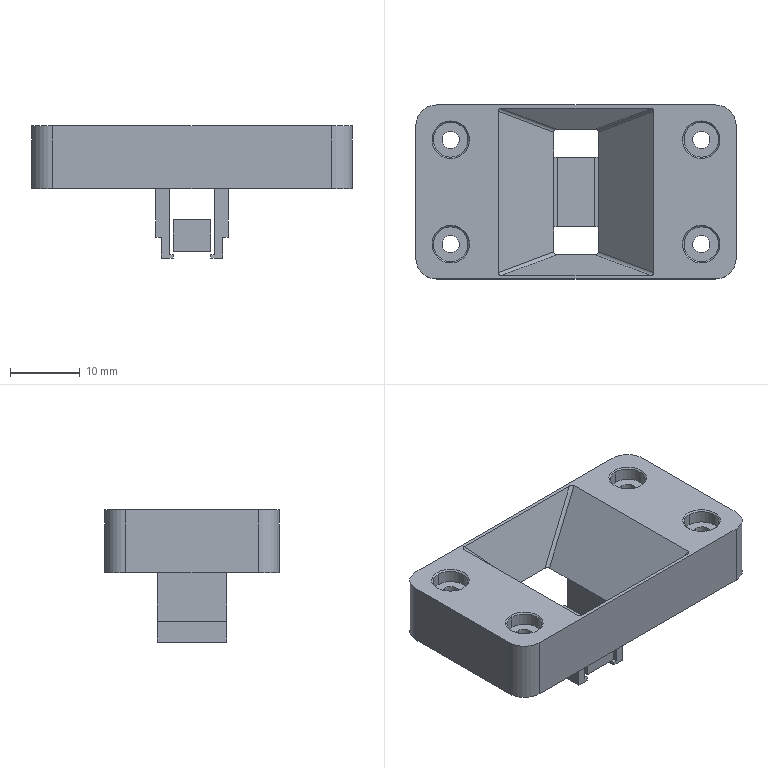NC program | NX | posted with a generic post | part box 46 x 25 x 19 mm
Lines 1 to 1574 of 3737:
N10 G17 G21 G94 G90
(FLOOR_WALL , TOOL : D63)
N12 T01 M6
N14 G54
N16 G17 G0 G90 X-60.5 Y0. S6500 M3
N18 G43 Z30. H1
N20 Z3.
N22 G94 G1 Z0. F1250.
N24 X-57.5
N26 X57.5
N28 X60.5
N30 Z3.
N32 G0 Z30.
N34 M5
(DRILLING_COPY_1 , TOOL : D6A45)
N36 T07 M6
N38 G54
N40 G17 G0 G90 X18. Y-7.5 S5000 M3
N42 G43 Z30. H7
N44 G94 G81 G98 Z-1. F250. R3.
N46 Y7.5
N48 X-18.
N50 Y-7.5
N52 G80
N54 G0 X-18. Y-7.5 Z30.
N56 M5
(DRILLING_COPY_COPY_1 , TOOL : 2.5ZT)
N58 T12 M6
N60 G54
N62 G17 G0 G90 X-18. Y7.5 S2000 M3
N64 G43 Z30. H12
N66 G94 G83 G98 Z-11.251 F120. Q2. R3.
N68 Y-7.5
N70 X18. Y7.5
N72 Y-7.5
N74 G80
N76 G0 X18. Y-7.5 Z30.
N78 M5
(ADAPTIVE_MILLING , TOOL : D10)
N80 T10 M6
N82 G54
N84 G17 G0 G90 X-33.697 Y-0.049 S9500 M3
N86 G43 Z30. H10
N88 Z-18.
N90 G94 G1 Z-19. F1000.
N92 X-32.34 Y-0.579 F3000.
N94 G3 X-31.05 Y-0.049 R1.015
N96 X-30.406 Y3.11 R9.424
N98 X-30.192 Y13.206 R193.319
N100 G2 X-27.283 Y17.541 R6.034
N102 X-21.613 Y19.34 R13.274
N104 X-12.124 Y19.68 R91.439
N106 G1 X-10.224 Y19.685
N108 X-7.224 Y19.689
N110 X0.376 Y19.69
N112 X23.276
N114 X23.376
N116 X23.476 Y19.686
N118 G2 X27.913 Y16.952 R5.88
N120 X29.811 Y11.32 R12.732
N122 X30.174 Y2.832 R75.409
N124 G1 X30.181 Y1.532
N126 X30.186 Y-0.468
N128 X30.189 Y-3.668
N130 X30.191 Y-12.268
N132 Y-12.768
N134 X30.19 Y-12.868
N136 X30.187 Y-12.967
N138 X30.182 Y-13.067
N140 X30.165 Y-13.267
N142 G2 X27.294 Y-17.52 R6.049
N144 X21.631 Y-19.334 R13.161
N146 X12.942 Y-19.676 R82.484
N148 G1 X11.342 Y-19.683
N150 X9.142 Y-19.687
N152 X5.242 Y-19.69
N154 X-17.158
N156 X-23.258
N158 X-23.358
N160 G2 X-27.727 Y-17.211 R5.74
N162 X-29.739 Y-11.833 R11.883
N164 X-30.084 Y-1.654 R57.601
N166 G3 X-29.419 Y10.621 R116.784
N168 G2 X-25.504 Y16.566 R7.722
N170 X-19.339 Y18.47 R15.631
N172 X-9.852 Y18.864 R87.436
N174 G1 X-8.252 Y18.872
N176 X-6.052 Y18.877
N178 X-2.552 Y18.88
N180 X7.048 Y18.882
N182 X20.548
N184 X20.648 Y18.881
N186 G2 X26.926 Y15.19 R7.564
N188 X28.962 Y8.865 R15.122
N190 X29.363 Y-0.521 R83.334
N192 X29.351 Y-10.72 R504.514
N194 X25.37 Y-16.621 R7.723
N196 X18.893 Y-18.518 R16.177
N198 X9.103 Y-18.868 R101.21
N200 G1 X7.603 Y-18.874
N202 X5.203 Y-18.878
N204 X0.903 Y-18.881
N206 X-20.497 Y-18.882
N208 X-20.697 Y-18.88
N210 X-20.897 Y-18.873
N212 G2 X-27.058 Y-14.981 R7.639
N214 X-29.004 Y-8.52 R15.779
N216 X-29.036 Y0.264 R43.131
N218 G3 X-28.648 Y8.654 R335.998
N220 G2 X-27.767 Y11.838 R8.866
N222 X-26.744 Y14.068 R8.11
N224 X-21.539 Y17.498 R8.456
N226 X-7.536 Y18.058 R139.726
N228 G1 X-5.536 Y18.065
N230 X-2.736 Y18.07
N232 X2.064 Y18.072
N234 X18.064 Y18.073
N236 X18.364 Y18.071
N238 X18.564 Y18.067
N240 G2 X21.765 Y17.44 R9.062
N242 X26.801 Y13.982 R8.383
N244 X28.147 Y9.526 R8.782
N246 X28.561 Y-3.864 R168.54
N248 X28.507 Y-8.962 R72.787
N250 X27.952 Y-11.228 R9.275
N252 X24.482 Y-16.301 R8.398
N254 X20.026 Y-17.647 R8.782
N256 X6.436 Y-18.062 R172.59
N258 G1 X4.036 Y-18.068
N260 X0.336 Y-18.072
N262 X-8.664 Y-18.073
N264 X-18.164
N266 X-18.364 Y-18.071
N268 X-18.564 Y-18.067
N270 G2 X-21.77 Y-17.439 R9.081
N272 X-26.801 Y-13.982 R8.381
N274 X-28.147 Y-9.526 R8.782
N276 X-28.15 Y1.332 R71.064
N278 G1 Y9.474
N280 X-28.147 Y9.526
N282 G2 X-27.746 Y11.905 R8.34
N284 G1 X-27.505 Y12.664
N286 X-27.133 Y13.371
N288 X-26.744 Y14.068
N290 X-26.241 Y14.688
N292 X-25.723 Y15.296
N294 X-25.109 Y15.806
N296 X-24.482 Y16.301
N298 X-23.78 Y16.681
N300 X-23.07 Y17.045
N302 X-22.307 Y17.281
N304 X-21.539 Y17.498
N306 X-20.026 Y17.647
N308 X-19.974 Y17.65
N310 X19.974
N312 X20.026 Y17.647
N314 G2 X21.831 Y17.42 R11.605
N316 G1 X22.5 Y17.221
N318 X23.164 Y17.005
N320 X23.871 Y16.633
N322 X24.568 Y16.244
N324 X25.188 Y15.741
N326 X25.796 Y15.223
N328 X26.306 Y14.609
N330 X26.801 Y13.982
N332 X27.181 Y13.28
N334 X27.545 Y12.57
N336 X27.781 Y11.807
N338 X27.998 Y11.039
N340 X28.147 Y9.526
N342 X28.15 Y9.474
N344 Y-9.474
N346 X28.147 Y-9.526
N348 G2 X27.949 Y-11.235 R72.543
N350 G1 X27.736 Y-11.952
N352 X27.505 Y-12.664
N354 X27.133 Y-13.371
N356 X26.744 Y-14.068
N358 X26.241 Y-14.688
N360 X25.723 Y-15.296
N362 X25.109 Y-15.806
N364 X24.482 Y-16.301
N366 X23.78 Y-16.681
N368 X23.07 Y-17.045
N370 X22.307 Y-17.281
N372 X21.539 Y-17.498
N374 X20.026 Y-17.647
N376 X19.974 Y-17.65
N378 X-19.974
N380 X-20.026 Y-17.647
N382 G2 X-21.831 Y-17.42 R11.605
N384 G1 X-22.5 Y-17.221
N386 X-23.164 Y-17.005
N388 X-23.871 Y-16.633
N390 X-24.568 Y-16.244
N392 X-25.188 Y-15.741
N394 X-25.796 Y-15.223
N396 X-26.306 Y-14.609
N398 X-26.801 Y-13.982
N400 X-27.181 Y-13.28
N402 X-27.545 Y-12.57
N404 X-27.781 Y-11.807
N406 X-27.998 Y-11.039
N408 X-28.147 Y-9.526
N410 X-28.15 Y-9.474
N412 Y1.426
N414 G3 X-29.013 Y2.425 R1.016
N416 G1 X-30.593 Y2.657
N418 Z-16.
N420 G0 Z30.
N422 M5
(ZLEVEL_PROFILE_COPY_COPY_1 , TOOL : D10JING)
N424 T11 M6
N426 G54
N428 G17 G0 G90 X-20.841 Y17.958 S9500 M3
N430 G43 Z30. H11
N432 Z-16.
N434 G94 G1 Z-19. F1200.
N436 G3 X-20. Y17.5 R1.
N438 G1 X20.
N440 G2 X28. Y9.5 R8.
N442 G1 Y-9.5
N444 G2 X20. Y-17.5 R8.
N446 G1 X-20.
N448 G2 X-28. Y-9.5 R8.
N450 G1 Y9.5
N452 G2 X-20. Y17.5 R8.
N454 G3 X-19.134 Y18. R1.
N456 G1 Z-16.
N458 G0 Z30.
N460 M5
(FIXED_CONTOUR , TOOL : D6)
N462 T06 M6
N464 G54
N466 G17 G0 G90 X8.757 Y2.485 S9500 M3
N468 G43 Z30. H6
N470 Z3.6
N472 G94 G1 Z0.438 F500.
N474 G3 X8.455 Y1.967 R0.6
N476 G1 X8.43 Y-6.253 Z0.409 F2500.
N478 X8.417 Y-8.89 Z0.395
N480 X8.419 Y-9.033 Z0.413
N482 X8.402 Y-9.043 Z0.444
N484 X4.433 Y-9.042 Z0.441
N486 X-5.767 Y-9.027 Z0.398
N488 X-8.137 Y-9.021 Z0.378
N490 X-8.38 Y-9.016 Z0.364
N492 X-8.377 Y-8.765 Z0.349
N494 X-8.331 Y6.648 Z0.298
N496 X-8.32 Y8.788 Z0.285
N498 X-8.318 Y8.996 Z0.303
N500 X-4.046 Y8.995 Z0.302
N502 X5.501 Y8.981 Z0.259
N504 X8.258 Y8.973 Z0.236
N506 X8.28 Y8.945 Z0.241
N508 X8.233 Y-6.326 Z0.188
N510 X8.221 Y-8.735 Z0.174
N512 X8.214 Y-8.947 Z0.166
N514 X4.808 Y-8.949 Z0.162
N516 X-6.007 Y-8.933 Z0.115
N518 X-8.145 Y-8.927 Z0.097
N520 X-8.181 Y-8.882 Z0.129
N522 X-8.134 Y6.844 Z0.076
N524 X-8.122 Y8.865 Z0.063
N526 X-8.069 Y8.903 Z0.025
N528 X-3.127 Y8.901 Z0.018
N530 X5.301 Y8.888 Z-0.021
N532 X8.03 Y8.878 Z-0.041
N534 X8.083 Y8.818 Z0.018
N536 X8.037 Y-6.324 Z-0.033
N538 X8.024 Y-8.757 Z-0.047
N540 X8.011 Y-8.805 Z-0.062
N542 X7.966 Y-8.854 Z-0.113
N544 X4.278 Y-8.855 Z-0.119
N546 X-5.897 Y-8.84 Z-0.165
N548 X-7.69 Y-8.835 Z-0.18
N550 X-7.913 Y-8.824 Z-0.173
N552 X-7.985 Y-8.745 Z-0.092
N554 X-7.939 Y6.483 Z-0.144
N556 X-7.927 Y8.714 Z-0.157
N558 X-7.834 Y8.809 Z-0.256
N560 X-3.07 Y8.807 Z-0.262
N562 X5.549 Y8.794 Z-0.303
N564 X7.782 Y8.786 Z-0.32
N566 X7.886 Y8.671 Z-0.202
N568 X7.841 Y-6.109 Z-0.253
N570 X7.829 Y-8.564 Z-0.267
N572 X7.818 Y-8.651 Z-0.279
N574 X7.705 Y-8.764 Z-0.393
N576 X2.414 Y-8.76 Z-0.406
N578 X-6.196 Y-8.745 Z-0.448
N580 X-7.54 Y-8.741 Z-0.46
N582 X-7.665 Y-8.73 Z-0.451
N584 X-7.789 Y-8.578 Z-0.312
N586 X-7.739 Y7.085 Z-0.368
N588 X-7.732 Y8.36 Z-0.376
N590 X-7.725 Y8.57 Z-0.384
N592 X-7.581 Y8.716 Z-0.536
N594 X-3.439 Y8.714 Z-0.541
N596 X5.431 Y8.7 Z-0.583
N598 X7.532 Y8.695 Z-0.598
N600 X7.668 Y8.546 Z-0.449
N602 X7.69 Y8.499 Z-0.423
N604 X7.645 Y-6.125 Z-0.475
N606 X7.632 Y-8.458 Z-0.488
N608 X7.618 Y-8.506 Z-0.505
N610 X7.476 Y-8.66 Z-0.664
N612 X7.217 Y-8.67 Z-0.674
N614 X0.537 Y-8.664 Z-0.692
N616 X-6.612 Y-8.651 Z-0.732
N618 X-7.266 Y-8.649 Z-0.738
N620 X-7.417 Y-8.638 Z-0.731
N622 X-7.555 Y-8.486 Z-0.575
N624 X-7.592 Y-8.426 Z-0.533
N626 X-7.542 Y7.225 Z-0.59
N628 X-7.535 Y8.385 Z-0.598
N630 X-7.518 Y8.432 Z-0.617
N632 X-7.379 Y8.583 Z-0.773
N634 X-7.336 Y8.623 Z-0.815
N636 X-3.098 Y8.621 Z-0.822
N638 X5.607 Y8.606 Z-0.865
N640 X7.165 Y8.603 Z-0.876
N642 X7.296 Y8.591 Z-0.867
N644 X7.444 Y8.427 Z-0.7
N646 X7.494 Y8.352 Z-0.644
N648 X7.448 Y-6.076 Z-0.695
N650 X7.435 Y-8.341 Z-0.71
N652 X7.214 Y-8.577 Z-0.952
N654 X0.101 Y-8.57 Z-0.976
N656 X-6.447 Y-8.557 Z-1.012
N658 X-7.125 Y-8.556 Z-1.017
N660 X-7.171 Y-8.543 Z-1.007
N662 X-7.3 Y-8.402 Z-0.862
N664 X-7.396 Y-8.282 Z-0.754
N666 X-7.344 Y7.325 Z-0.812
N668 X-7.339 Y8.248 Z-0.818
N670 X-7.206 Y8.407 Z-0.968
N672 X-7.084 Y8.53 Z-1.095
N674 X-3.316 Y8.528 Z-1.101
N676 X5.401 Y8.513 Z-1.144
N678 X7.035 Y8.51 Z-1.155
N680 X7.298 Y8.222 Z-0.865
N682 X7.25 Y-6.314 Z-0.918
N684 X7.239 Y-8.191 Z-0.931
N686 X7.097 Y-8.346 Z-1.09
N688 X6.961 Y-8.484 Z-1.232
N690 X-1.38 Y-8.474 Z-1.262
N692 X-6.909 Y-8.463 Z-1.296
N694 X-7.166 Y-8.182 Z-1.013
N696 X-7.2 Y-8.132 Z-0.975
N698 X-7.147 Y7.464 Z-1.035
N700 X-7.143 Y8.112 Z-1.039
N702 X-6.86 Y8.418 Z-1.357
N704 X-6.808 Y8.436 Z-1.375
N706 X-2.814 Y8.434 Z-1.384
N708 X5.435 Y8.42 Z-1.425
N710 X6.792 Y8.414 Z-1.434
N712 X7.074 Y8.102 Z-1.117
N714 X7.101 Y8.049 Z-1.086
N716 X7.055 Y-5.998 Z-1.137
N718 X7.043 Y-8.04 Z-1.151
N720 X6.766 Y-8.342 Z-1.463
N722 X6.703 Y-8.391 Z-1.512
N724 X-1.526 Y-8.38 Z-1.544
N726 X-6.462 Y-8.37 Z-1.574
N728 X-6.672 Y-8.362 Z-1.568
N730 X-6.94 Y-8.065 Z-1.267
N732 X-7.004 Y-7.984 Z-1.195
N734 X-6.951 Y7.324 Z-1.255
N736 X-6.947 Y7.961 Z-1.259
N738 X-6.669 Y8.263 Z-1.572
N740 X-6.587 Y8.343 Z-1.655
N742 X-2.976 Y8.34 Z-1.663
N744 X5.308 Y8.326 Z-1.705
N746 X6.498 Y8.323 Z-1.714
N748 X6.556 Y8.308 Z-1.699
N750 X6.905 Y7.922 Z-1.307
N752 X6.858 Y-6.073 Z-1.359
N754 X6.849 Y-7.739 Z-1.369
N756 X6.838 Y-7.9 Z-1.382
N758 X6.545 Y-8.22 Z-1.712
N760 X6.462 Y-8.298 Z-1.791
N762 X-1.462 Y-8.287 Z-1.824
N764 X-6.202 Y-8.277 Z-1.852
N766 X-6.428 Y-8.264 Z-1.843
N768 X-6.67 Y-7.997 Z-1.571
N770 X-6.807 Y-7.837 Z-1.416
N772 X-6.755 Y7.16 Z-1.475
N774 X-6.752 Y7.631 Z-1.478
N776 X-6.745 Y7.817 Z-1.486
N778 X-6.347 Y8.249 Z-1.934
N780 X-2.561 Y8.246 Z-1.945
N782 X5.253 Y8.233 Z-1.985
N784 X6.064 Y8.231 Z-1.991
N786 X6.301 Y8.223 Z-1.986
N788 X6.709 Y7.772 Z-1.528
N790 X6.66 Y-6.35 Z-1.582
N792 X6.653 Y-7.59 Z-1.59
N794 X6.645 Y-7.746 Z-1.598
N796 X6.36 Y-8.056 Z-1.919
N798 X6.215 Y-8.204 Z-2.071
N800 X-2.643 Y-8.191 Z-2.111
N802 X-5.955 Y-8.184 Z-2.131
N804 X-6.175 Y-8.179 Z-2.128
N806 X-6.558 Y-7.753 Z-1.696
N808 X-6.611 Y-7.681 Z-1.637
N810 X-6.559 Y6.99 Z-1.695
N812 X-6.556 Y7.471 Z-1.699
N814 X-6.549 Y7.667 Z-1.707
N816 X-6.132 Y8.119 Z-2.176
N818 X-6.074 Y8.157 Z-2.214
N820 X-1.07 Y8.151 Z-2.232
N822 X5.446 Y8.139 Z-2.268
N824 X5.872 Y8.138 Z-2.271
N826 X6.056 Y8.126 Z-2.261
N828 X6.441 Y7.701 Z-1.828
N830 X6.512 Y7.604 Z-1.749
N832 X6.465 Y-6.029 Z-1.802
N834 X6.456 Y-7.588 Z-1.811
N836 X5.972 Y-8.11 Z-2.353
N838 X-1.594 Y-8.1 Z-2.385
N840 X-5.916 Y-8.091 Z-2.41
N842 X-6.151 Y-7.837 Z-2.155
N844 X-6.29 Y-7.682 Z-1.998
N846 X-6.415 Y-7.531 Z-1.858
N848 X-6.362 Y7. Z-1.917
N850 X-6.359 Y7.509 Z-1.92
N852 X-5.851 Y8.06 Z-2.492
N854 X-1.703 Y8.058 Z-2.509
N856 X5.307 Y8.045 Z-2.547
N858 X5.708 Y8.044 Z-2.551
N860 X5.809 Y8.032 Z-2.539
N862 X6.306 Y7.482 Z-1.98
N864 X6.315 Y7.225 Z-1.97
N866 X6.268 Y-6.118 Z-2.023
N868 X6.261 Y-7.25 Z-2.031
N870 X6.256 Y-7.443 Z-2.037
N872 X5.857 Y-7.875 Z-2.485
N874 X5.711 Y-8.017 Z-2.632
N876 X-3.184 Y-8.003 Z-2.675
N878 X-5.604 Y-7.998 Z-2.689
N880 X-5.685 Y-7.987 Z-2.679
N882 X-6.172 Y-7.446 Z-2.131
N884 X-6.219 Y-7.374 Z-2.078
N886 X-6.165 Y7.165 Z-2.14
N888 X-6.161 Y7.361 Z-2.144
N890 X-5.613 Y7.954 Z-2.76
N892 X-5.562 Y7.97 Z-2.774
N894 X4.043 Y7.955 Z-2.818
N896 X5.524 Y7.951 Z-2.83
N898 X5.575 Y7.924 Z-2.803
N900 X6.058 Y7.39 Z-2.26
N902 X6.12 Y7.303 Z-2.19
N904 X6.071 Y-6.062 Z-2.244
N906 X6.065 Y-7.09 Z-2.251
N908 X6.054 Y-7.298 Z-2.264
N910 X5.514 Y-7.883 Z-2.871
N912 X5.458 Y-7.923 Z-2.913
N914 X-2.94 Y-7.91 Z-2.954
N916 X-5.185 Y-7.906 Z-2.967
N918 X-5.434 Y-7.898 Z-2.962
N920 X-6.023 Y-7.243 Z-2.299
N922 X-5.969 Y7.02 Z-2.36
N924 X-5.965 Y7.21 Z-2.364
N926 X-5.352 Y7.875 Z-3.054
N928 X4.947 Y7.859 Z-3.107
N930 X5.304 Y7.855
N932 X5.923 Y7.166 Z-2.411
N934 X5.874 Y-6.159 Z-2.466
N936 X5.868 Y-7.108 Z-2.473
N938 X5.858 Y-7.148 Z-2.484
N940 X5.255 Y-7.799 Z-3.162
N942 X5.217 Y-7.83 Z-3.193
N944 X-4.705 Y-7.813 Z-3.245
N946 X-4.972 Y-7.812 Z-3.247
N948 X-5.187 Y-7.803 Z-3.239
N950 X-5.826 Y-7.092 Z-2.52
N952 X-5.773 Y6.869 Z-2.58
N954 X-5.765 Y7.065 Z-2.59
N956 X-5.105 Y7.78 Z-3.331
N958 X-3.502 Y7.781 Z-3.34
N960 X4.795 Y7.766 Z-3.386
N962 X5.059 Y7.758 Z-3.383
N964 X5.587 Y7.175 Z-2.789
N966 X5.727 Y7.003 Z-2.632
N968 X5.677 Y-6.136 Z-2.688
N970 X5.673 Y-6.755 Z-2.692
N972 X5.662 Y-6.997 Z-2.705
N974 X5.058 Y-7.649 Z-3.383
N976 X4.961 Y-7.736 Z-3.475
N978 X-2.963 Y-7.723 Z-3.516
N980 X-4.752 Y-7.719 Z-3.527
N982 X-4.938 Y-7.71 Z-3.519
N984 X-5.488 Y-7.101 Z-2.901
N986 X-5.63 Y-6.931 Z-2.741
N988 X-5.576 Y6.847 Z-2.802
N990 X-5.566 Y6.917 Z-2.813
N992 X-4.985 Y7.547 Z-3.466
N994 X-4.845 Y7.69 Z-3.613
N996 X4.729 Y7.672 Z-3.666
N998 X4.816 Y7.66 Z-3.657
N1000 X5.493 Y6.912 Z-2.895
N1002 X5.531 Y6.85 Z-2.853
N1004 X5.479 Y-6.257 Z-2.91
N1006 X5.476 Y-6.836 Z-2.914
N1008 X4.826 Y-7.537 Z-3.645
N1010 X4.707 Y-7.643 Z-3.756
N1012 X-3.068 Y-7.629 Z-3.797
N1014 X-4.47 Y-7.626 Z-3.806
N1016 X-4.691 Y-7.616 Z-3.797
N1018 X-5.295 Y-6.947 Z-3.118
N1020 X-5.434 Y-6.784 Z-2.961
N1022 X-5.381 Y6.522 Z-3.021
N1024 X-5.372 Y6.764 Z-3.031
N1026 X-4.603 Y7.597 Z-3.894
N1028 X4.407 Y7.578 Z-3.944
N1030 X4.564 Y7.57 Z-3.94
N1032 X5.334 Y6.719 Z-3.073
N1034 X5.284 Y-6.02 Z-3.13
N1036 X5.282 Y-6.391 Z-3.132
N1038 X5.272 Y-6.693 Z-3.143
N1040 X4.521 Y-7.502 Z-3.987
N1042 X4.461 Y-7.549 Z-4.036
N1044 X-4.202 Y-7.533 Z-4.085
N1046 X-4.444 Y-7.522 Z-4.075
N1048 X-5.221 Y-6.662 Z-3.201
N1050 X-5.238 Y-6.609 Z-3.182
N1052 X-5.184 Y6.384 Z-3.242
N1054 X-5.177 Y6.612 Z-3.251
N1056 X-4.47 Y7.378 Z-4.045
N1058 X-4.344 Y7.503 Z-4.175
N1060 X4.229 Y7.484 Z-4.224
N1062 X4.323 Y7.469 Z-4.211
N1064 X5.048 Y6.669 Z-3.396
N1066 X5.138 Y6.549 Z-3.294
N1068 X5.086 Y-6.08 Z-3.352
N1070 X5.084 Y-6.423 Z-3.354
N1072 X5.077 Y-6.54 Z-3.362
N1074 X4.225 Y-7.456 Z-4.316
N1076 X-4.051 Y-7.44 Z-4.365
N1078 X-4.196 Y-7.428 Z-4.354
N1080 X-5.041 Y-6.492 Z-3.403
N1082 X-4.987 Y6.406 Z-3.464
N1084 X-4.982 Y6.46 Z-3.47
N1086 X-4.216 Y7.289 Z-4.331
N1088 X-4.093 Y7.41 Z-4.455
N1090 X4.048 Y7.393 Z-4.503
N1092 X4.183 Y7.258 Z-4.368
N1094 X4.942 Y6.413 Z-3.515
N1096 X4.888 Y-6.241 Z-3.575
N1098 Y-6.382 Z-3.576
N1100 X3.994 Y-7.344 Z-4.58
N1102 X3.951 Y-7.362 Z-4.598
N1104 X-3.857 Y-7.346 Z-4.644
N1106 X-3.945 Y-7.338 Z-4.637
N1108 X-4.845 Y-6.338 Z-3.624
N1110 X-4.791 Y6.305 Z-3.685
N1112 X-3.909 Y7.257 Z-4.677
N1114 X-3.833 Y7.316 Z-4.737
N1116 X3.796 Y7.3 Z-4.783
N1118 X3.926 Y7.177 Z-4.658
N1120 X4.723 Y6.293 Z-3.762
N1122 X4.745 Y6.244 Z-3.736
N1124 X4.692 Y-6.156 Z-3.796
N1126 X4.685 Y-6.238 Z-3.804
N1128 X3.745 Y-7.25 Z-4.86
N1130 X3.72 Y-7.268 Z-4.879
N1132 X-3.471 Y-7.254 Z-4.923
N1134 X-3.698 Y-7.243 Z-4.915
N1136 X-4.506 Y-6.35 Z-4.005
N1138 X-4.649 Y-6.181 Z-3.845
N1140 X-4.595 Y5.904 Z-3.905
N1142 X-4.587 Y6.162 Z-3.914
N1144 X-3.703 Y7.115 Z-4.908
N1146 X-3.599 Y7.222 Z-5.019
N1148 X3.312 Y7.208 Z-5.061
N1150 X3.571 Y7.199 Z-5.056
N1152 X4.388 Y6.296 Z-4.138
N1154 X4.549 Y6.099 Z-3.957
N1156 X4.495 Y-6.073 Z-4.017
N1158 X4.14 Y-6.462 Z-4.416
N1160 X3.571 Y-7.075 Z-5.056
N1162 X3.464 Y-7.175 Z-5.16
N1164 X-3.264 Y-7.16 Z-5.203
N1166 X-3.448 Y-7.152 Z-5.196
N1168 X-4.344 Y-6.161 Z-4.187
N1170 X-4.452 Y-6.031 Z-4.066
N1172 X-4.398 Y6.004 Z-4.127
N1174 X-3.379 Y7.099 Z-5.273
N1176 X-3.334 Y7.128 Z-5.299
N1178 X3.193 Y7.114 Z-5.341
N1180 X3.32 Y7.109 Z-5.339
N1182 X4.184 Y6.154 Z-4.368
N1184 X4.353 Y5.956 Z-4.178
N1186 X4.3 Y-5.844 Z-4.237
N1188 X4.288 Y-5.941 Z-4.25
N1190 X3.235 Y-7.073 Z-5.434
N1192 X2.995 Y-7.08 Z-5.443
N1194 X-3.043 Y-7.067 Z-5.482
N1196 X-3.202 Y-7.056 Z-5.472
N1198 X-4.243 Y-5.905 Z-4.301
N1200 X-4.256 Y-5.842 Z-4.287
N1202 X-4.201 Y5.854 Z-4.348
N1204 X-3.105 Y7.032 Z-5.581
N1206 X3.004 Y7.021 Z-5.621
N1208 X3.076 Y7.011 Z-5.613
N1210 X4.051 Y5.932 Z-4.516
N1212 X4.156 Y5.803 Z-4.399
N1214 X4.103 Y-5.777 Z-4.458
N1216 X2.979 Y-6.985 Z-5.722
N1218 X-2.932 Y-6.974 Z-5.761
N1220 X-3.082 Y-6.821 Z-5.607
N1222 X-3.905 Y-5.911 Z-4.681
N1224 X-4.06 Y-5.721 Z-4.507
N1226 X-4.006 Y5.43 Z-4.567
N1228 X-3.998 Y5.711 Z-4.577
N1230 X-2.881 Y6.91 Z-5.833
N1232 X-2.812 Y6.94 Z-5.863
N1234 X2.776 Y6.928 Z-5.9
N1236 X2.833 Y6.912 Z-5.887
N1238 X3.855 Y5.782 Z-4.737
N1240 X3.96 Y5.649 Z-4.619
N1242 X3.907 Y-5.626 Z-4.679
N1244 X2.725 Y-6.893 Z-6.004
N1246 X-2.457 Y-6.881 Z-6.04
N1248 X-2.705 Y-6.87 Z-6.031
N1250 X-3.863 Y-5.589 Z-4.728
N1252 X-3.81 Y5.264 Z-4.788
N1254 X-3.8 Y5.562 Z-4.8
N1256 X-2.605 Y6.843 Z-6.144
N1258 X2.357 Y6.835 Z-6.179
N1260 X2.577 Y6.828 Z-6.175
N1262 X3.707 Y5.577 Z-4.903
N1264 X3.763 Y5.502 Z-4.84
N1266 X3.711 Y-5.475 Z-4.899
N1268 X2.476 Y-6.799 Z-6.285
N1270 X-2.263 Y-6.788 Z-6.319
N1272 X-2.457 Y-6.777 Z-6.31
N1274 X-3.507 Y-5.615 Z-5.129
N1276 X-3.667 Y-5.421 Z-4.949
N1278 X-3.612 Y5.344 Z-5.011
N1280 X-3.601 Y5.414 Z-5.023
N1282 X-2.432 Y6.667 Z-6.338
N1284 X-2.334 Y6.752 Z-6.427
N1286 X2.251 Y6.742 Z-6.459
N1288 X2.325 Y6.737 Z-6.458
N1290 X3.403 Y5.546 Z-5.246
N1292 X3.567 Y5.358 Z-5.061
N1294 X3.516 Y-5.1 Z-5.118
N1296 X3.507 Y-5.332 Z-5.128
N1298 X2.302 Y-6.627 Z-6.484
N1300 X2.205 Y-6.706 Z-6.567
N1302 X-2.07 Y-6.695 Z-6.599
N1304 X-2.208 Y-6.685 Z-6.59
N1306 X-3.471 Y-5.286 Z-5.17
N1308 X-3.416 Y5.225 Z-5.232
N1310 X-3.393 Y5.276 Z-5.258
N1312 X-2.215 Y6.538 Z-6.583
N1314 X-2.085 Y6.658 Z-6.71
N1316 X1.946 Y6.649 Z-6.738
N1318 X2.078 Y6.643 Z-6.735
N1320 X3.212 Y5.389 Z-5.461
N1322 X3.371 Y5.194 Z-5.282
N1324 X3.319 Y-4.974 Z-5.339
N1326 X3.31 Y-5.182 Z-5.35
N1328 X1.986 Y-6.601 Z-6.839
N1330 X1.754 Y-6.611 Z-6.85
N1332 X-1.934 Y-6.602 Z-6.879
N1334 X-2.064 Y-6.477 Z-6.753
N1336 X-3.15 Y-5.273 Z-5.531
N1338 X-3.274 Y-5.126 Z-5.391
N1340 X-3.219 Y5.046 Z-5.453
N1342 X-3.212 Y5.108 Z-5.461
N1344 X-1.853 Y6.559 Z-6.989
N1346 X-1.211 Y6.563 Z-6.996
N1348 X1.777 Y6.555 Z-7.018
N1350 X1.838 Y6.541 Z-7.006
N1352 X2.994 Y5.264 Z-5.706
N1354 X3.174 Y5.044 Z-5.503
N1356 X3.122 Y-4.933 Z-5.561
N1358 X3.113 Y-5.03 Z-5.572
N1360 X1.726 Y-6.516 Z-7.131
N1362 X-1.578 Y-6.509 Z-7.157
N1364 X-1.713 Y-6.496 Z-7.147
N1366 X-3.006 Y-5.064 Z-5.692
N1368 X-3.078 Y-4.973 Z-5.612
N1370 X-3.025 Y4.618 Z-5.672
N1372 X-3.015 Y4.957 Z-5.682
N1374 X-1.644 Y6.421 Z-7.225
N1376 X-1.598 Y6.468 Z-7.276
N1378 X0.595 Y6.465 Z-7.29
N1380 X1.575 Y6.462 Z-7.299
N1382 X2.966 Y4.925 Z-5.738
N1384 X2.977 Y4.864 Z-5.724
N1386 X2.926 Y-4.691 Z-5.782
N1388 X2.916 Y-4.88 Z-5.793
N1390 X1.495 Y-6.401 Z-7.391
N1392 X1.461 Y-6.423 Z-7.414
N1394 X-1.3 Y-6.416 Z-7.436
N1396 X-1.464 Y-6.403 Z-7.428
N1398 X-2.714 Y-5.02 Z-6.022
N1400 X-2.881 Y-4.823 Z-5.833
N1402 X-2.826 Y4.798 Z-5.895
N1404 X-1.458 Y6.261 Z-7.434
N1406 X-1.333 Y6.375 Z-7.558
N1408 X1.134 Y6.37 Z-7.575
N1410 X1.336 Y6.358 Z-7.57
N1412 X2.122 Y5.494 Z-6.687
N1414 X2.604 Y4.959 Z-6.144
N1416 X2.781 Y4.752 Z-5.945
N1418 X2.729 Y-4.576 Z-6.003
N1420 X2.723 Y-4.726 Z-6.01
N1422 X1.342 Y-6.206 Z-7.564
N1424 X1.211 Y-6.328 Z-7.699
N1426 X-0.584 Y-6.324 Z-7.71
N1428 X-1.018 Y-6.323 Z-7.714
N1430 X-1.211 Y-6.311 Z-7.712
N1432 X-1.49 Y-6.01 Z-7.399
N1434 X-2.668 Y-4.702 Z-6.073
N1436 X-2.685 Y-4.649 Z-6.054
N1438 X-2.63 Y4.647 Z-6.116
N1440 X-1.156 Y6.218 Z-7.774
N1442 X-1.079 Y6.281 Z-7.842
N1444 X-0.126 Y6.279 Z-7.845
N1446 X0.875 Y6.277 Z-7.854
N1448 X1.085 Y6.266 Z-7.853
N1450 X1.306 Y6.029 Z-7.604
N1452 X2.519 Y4.685 Z-6.24
N1454 X2.585 Y4.592 Z-6.166
N1456 X2.532 Y-4.568 Z-6.225
N1458 X1.087 Y-6.116 Z-7.85
N1460 X0.95 Y-6.233 Z-7.985
N1462 X0.738 Y-6.235 Z-7.979
N1464 X-0.819 Y-6.23 Z-7.993
N1466 X-0.961 Y-6.216
N1468 X-1.073 Y-6.103 Z-7.867
N1470 X-2.41 Y-4.619 Z-6.364
N1472 X-2.488 Y-4.516 Z-6.275
N1474 X-2.433 Y4.496 Z-6.337
N1476 X-0.958 Y6.071 Z-7.997
N1478 X-0.835 Y6.185 Z-8.128
N1480 X-0.485 Y6.187 Z-8.123
N1482 X0.712 Y6.183 Z-8.133
N1484 X0.831 Y6.175 Z-8.138
N1486 X0.928 Y6.08 Z-8.03
N1488 X2.388 Y4.461 Z-6.387
N1490 X2.337 Y-4.091 Z-6.444
N1492 X2.329 Y-4.424 Z-6.454
N1494 X0.823 Y-6.035 Z-8.147
N1496 X0.698 Y-6.136 Z-8.275
N1498 X0.51 Y-6.141 Z-8.262
N1500 X-0.561 Y-6.137 Z-8.272
N1502 X-0.708 Y-6.121 Z-8.278
N1504 X-0.835 Y-6.001 Z-8.135
N1506 X-2.292 Y-4.381 Z-6.496
N1508 X-2.236 Y4.344 Z-6.559
N1510 X-0.691 Y5.994 Z-8.298
N1512 X-0.57 Y6.091 Z-8.41
N1514 X-0.177 Y6.092 Z-8.406
N1516 X0.38 Y6.091 Z-8.411
N1518 X0.577 Y6.084 Z-8.424
N1520 X0.691 Y5.974 Z-8.295
N1522 X2. Y4.522 Z-6.823
N1524 X2.191 Y4.294 Z-6.608
N1526 X2.139 Y-4.225 Z-6.667
N1528 X2.132 Y-4.273 Z-6.675
N1530 X0.561 Y-5.952 Z-8.442
N1532 X0.468 Y-6.027 Z-8.547
N1534 X0.409 Y-6.04 Z-8.562
N1536 X0.218 Y-6.046 Z-8.545
N1538 X-0.306 Y-6.044 Z-8.55
N1540 X-0.435 Y-6.035 Z-8.578
N1542 X-0.538 Y-5.962 Z-8.469
N1544 X-2.029 Y-4.303 Z-6.792
N1546 X-2.095 Y-4.216 Z-6.717
N1548 X-2.04 Y4.193 Z-6.78
N1550 X-0.424 Y5.912 Z-8.597
N1552 X-0.319 Y5.996 Z-8.696
N1554 X-0.142 Y5.999 Z-8.687
N1556 X0.239 Y5.998 Z-8.691
N1558 X0.334 Y5.981 Z-8.697
N1560 X0.453 Y5.871 Z-8.564
N1562 X1.841 Y4.33 Z-7.003
N1564 X1.995 Y4.142 Z-6.829
N1566 X1.942 Y-4.058 Z-6.888
N1568 X1.931 Y-4.127 Z-6.901
N1570 X0.369 Y-5.794 Z-8.658
N1572 X0.248 Y-5.914 Z-8.794
N1574 X0.186 Y-5.936 Z-8.864
N1576 X0.019 Y-5.952 Z-8.828
N1578 X-0.179 Y-5.938 Z-8.871
N1580 X-0.265 Y-5.897 Z-8.776
N1582 X-1.704 Y-4.296 Z-7.157
N1584 X-1.899 Y-4.06 Z-6.938
N1586 X-1.843 Y4.041 Z-7.001
N1588 X-0.196 Y5.796 Z-8.854
N1590 X-0.065 Y5.9 Z-8.984
N1592 X0.039 Y5.905 Z-8.97
N1594 X0.079 Y5.887 Z-8.983
N1596 X0.194 Y5.789 Z-8.854
N1598 X1.774 Y4.034 Z-7.077
N1600 X1.798 Y3.985 Z-7.051
N1602 X1.745 Y-3.9 Z-7.11
N1604 X1.734 Y-3.975 Z-7.122
N1606 X0.084 Y-5.733 Z-8.978
N1608 X0.009 Y-5.783 Z-9.062
N1610 X-0.048 Y-5.771 Z-9.02
N1612 X-1.702 Y-3.925 Z-7.159
N1614 X-1.646 Y3.89 Z-7.223
N1616 X-0.114 Y5.519 Z-8.946
N1618 X0.008 Y5.629 Z-9.064
N1620 X1.602 Y3.856 Z-7.272
N1622 X1.549 Y-3.529 Z-7.331
N1624 X1.541 Y-3.819 Z-7.34
N1626 X0.077 Y-5.376 Z-8.986
N1628 X-0.008 Y-5.449 Z-9.065
N1630 X-1.432 Y-3.859 Z-7.463
N1632 X-1.506 Y-3.767 Z-7.38
N1634 X-1.448 Y3.738 Z-7.445
N1636 X-0.007 Y5.267 Z-9.066
N1638 X0.108 Y5.153 Z-8.951
N1640 X1.306 Y3.816 Z-7.604
N1642 X1.405 Y3.688 Z-7.493
N1644 X1.35 Y-3.521 Z-7.555
N1646 X1.343 Y-3.666 Z-7.562
N1648 X-0.001 Y-5.09 Z-9.073
N1650 X-1.176 Y-3.775 Z-7.751
N1652 X-1.31 Y-3.616 Z-7.601
N1654 X-1.252 Y3.362 Z-7.666
N1656 X-1.241 Y3.594 Z-7.678
N1658 X-0.031 Y4.875 Z-9.039
N1660 X0.004 Y4.902 Z-9.069
N1662 X1.061 Y3.72 Z-7.88
N1664 X1.209 Y3.538 Z-7.713
N1666 X1.151 Y-3.37 Z-7.779
N1668 X1.143 Y-3.514 Z-7.787
N1670 X-0.001 Y-4.723 Z-9.073
N1672 X-1.05 Y-3.546 Z-7.893
N1674 X-1.113 Y-3.458 Z-7.822
N1676 X-1.051 Y3.399 Z-7.892
N1678 X-1.035 Y3.448 Z-7.91
N1680 X-0.068 Y4.469 Z-8.998
N1682 X0.004 Y4.535 Z-9.069
N1684 X0.933 Y3.492 Z-8.023
N1686 X1.012 Y3.388 Z-7.934
N1688 X0.953 Y-3.068 Z-8.001
N1690 X0.943 Y-3.362 Z-8.012
N1692 X-0.001 Y-4.355 Z-9.073
N1694 X-0.803 Y-3.452 Z-8.17
N1696 X-0.917 Y-3.307 Z-8.043
N1698 X-0.853 Y3.177 Z-8.115
N1700 X-0.847 Y3.283 Z-8.121
N1702 X-0.061 Y4.109 Z-9.006
N1704 X0.007 Y4.164 Z-9.065
N1706 X0.816 Y3.252 Z-8.155
N1708 X0.752 Y-2.997 Z-8.227
N1710 X0.739 Y-3.211 Z-8.241
N1712 X-0.001 Y-3.987 Z-9.073
N1714 X-0.601 Y-3.309 Z-8.399
N1716 X-0.721 Y-3.161 Z-8.264
N1718 X-0.652 Y3.078 Z-8.341
N1720 X-0.639 Y3.137 Z-8.355
N1722 X-0.024 Y3.78 Z-9.048
N1724 X0.005 Y3.798 Z-9.067
N1726 X0.568 Y3.159 Z-8.434
N1728 X0.62 Y3.084 Z-8.376
N1730 X0.55 Y-2.939 Z-8.454
N1732 X0.544 Y-3.05 Z-8.461
N1734 X0.092 Y-3.524 Z-8.969
N1736 X-0.006 Y-3.612 Z-9.067
N1738 X-0.447 Y-3.11 Z-8.571
N1740 X-0.524 Y-3.012 Z-8.484
N1742 X-0.453 Y2.749 Z-8.565
N1744 X-0.444 Y2.976 Z-8.575
N1746 X-0.073 Y3.359 Z-8.992
N1748 X0.007 Y3.426 Z-9.065
N1750 X0.42 Y2.953 Z-8.601
N1752 X0.409 Y1.819 Z-8.612
N1754 X0.348 Y-2.741 Z-8.681
N1756 X0.343 Y-2.892 Z-8.687
N1758 X-0.002 Y-3.246 Z-9.073
N1760 X-0.31 Y-2.892 Z-8.725
N1762 X-0.328 Y-2.846 Z-8.706
N1764 X-0.251 Y2.565 Z-8.792
N1766 X-0.242 Y2.819 Z-8.802
N1768 X0.003 Y3.06 Z-9.069
N1770 X0.226 Y2.783 Z-8.818
N1772 X0.142 Y-2.73 Z-8.913
N1774 X-0.007 Y-2.867 Z-9.066
N1776 X-0.131 Y-2.71 Z-8.927
N1778 X-0.052 Y2.124 Z-9.016
N1780 X-0.04 Y2.659 Z-9.029
N1782 X0.006 Y2.682 Z-9.066
N1784 X0.029 Y2.617 Z-9.04
N1786 X0.019 Y1.965 Z-9.052
N1788 Y-1.869 Z-9.051
N1790 X0.01 Y-2.65 Z-9.062
N1792 X-0.022 Y-2.636 Z-9.05
N1794 X-0.055 Y-2.601
N1796 X-0.081 Y-2.642
N1798 Z-3.6
N1800 G0 Z30.
N1802 M5
(ZLEVEL_PROFILE , TOOL : D4)
N1804 T04 M6
N1806 G54
N1808 G17 G0 G90 X0.292 Y6.9 S9500 M3
N1810 G43 Z30. H4
N1812 Z-7.5
N1814 G94 G1 X-1.1 Z-7.573 F800.
N1816 Y-6.9 Z-8.296
N1818 X1.1 Z-8.411
N1820 Y6.9 Z-9.135
N1822 X-1.1 Z-9.25
N1824 Y-6.9 F2000.
N1826 X1.1
N1828 Y6.9
N1830 X-1.1
N1832 Y-6.861 Z-9.49
N1834 X-0.999 Y-6.9 Z-9.493
N1836 X-0.578 Z-9.5
N1838 X1.1
N1840 Y6.9
N1842 X-1.1
N1844 Y-6.861 Z-9.74
N1846 X-0.999 Y-6.9 Z-9.743
N1848 X-0.578 Z-9.75
N1850 X1.1
N1852 Y6.9
N1854 X-1.1
N1856 Y-6.861 Z-9.99
N1858 X-0.999 Y-6.9 Z-9.993
N1860 X-0.578 Z-10.
N1862 X1.1
N1864 Y6.9
N1866 X-1.1
N1868 Y-6.861 Z-10.24
N1870 X-0.999 Y-6.9 Z-10.243
N1872 X-0.578 Z-10.25
N1874 X1.1
N1876 Y6.9
N1878 X-1.1
N1880 Y-6.861 Z-10.49
N1882 X-0.999 Y-6.9 Z-10.493
N1884 X-0.578 Z-10.5
N1886 X1.1
N1888 Y6.9
N1890 X-1.1
N1892 Y-6.861 Z-10.74
N1894 X-0.999 Y-6.9 Z-10.743
N1896 X-0.578 Z-10.75
N1898 X1.1
N1900 Y6.9
N1902 X-1.1
N1904 Y-6.861 Z-10.99
N1906 X-0.999 Y-6.9 Z-10.993
N1908 X-0.578 Z-11.
N1910 X1.1
N1912 Y6.9
N1914 X-1.1
N1916 Y-6.861 Z-11.24
N1918 X-0.999 Y-6.9 Z-11.243
N1920 X-0.578 Z-11.25
N1922 X1.1
N1924 Y6.9
N1926 X-1.1
N1928 Y-6.861 Z-11.49
N1930 X-0.999 Y-6.9 Z-11.493
N1932 X-0.578 Z-11.5
N1934 X1.1
N1936 Y6.9
N1938 X-1.1
N1940 Y-6.861 Z-11.74
N1942 X-0.999 Y-6.9 Z-11.743
N1944 X-0.578 Z-11.75
N1946 X1.1
N1948 Y6.9
N1950 X-1.1
N1952 Y-6.861 Z-11.99
N1954 X-0.999 Y-6.9 Z-11.993
N1956 X-0.578 Z-12.
N1958 X1.1
N1960 Y6.9
N1962 X-1.1
N1964 Y-6.861 Z-12.24
N1966 X-0.999 Y-6.9 Z-12.243
N1968 X-0.578 Z-12.25
N1970 X1.1
N1972 Y6.9
N1974 X-1.1
N1976 Y-6.861 Z-12.49
N1978 X-0.999 Y-6.9 Z-12.493
N1980 X-0.578 Z-12.5
N1982 X1.1
N1984 Y6.9
N1986 X-1.1
N1988 Y-6.861 Z-12.74
N1990 X-0.999 Y-6.9 Z-12.743
N1992 X-0.578 Z-12.75
N1994 X1.1
N1996 Y6.9
N1998 X-1.1
N2000 Y-6.861 Z-12.99
N2002 X-0.999 Y-6.9 Z-12.993
N2004 X-0.578 Z-13.
N2006 X1.1
N2008 Y6.9
N2010 X-1.1
N2012 Y-6.861 Z-13.24
N2014 X-0.999 Y-6.9 Z-13.243
N2016 X-0.578 Z-13.25
N2018 X1.1
N2020 Y6.9
N2022 X-1.1
N2024 Y-6.861 Z-13.49
N2026 X-0.999 Y-6.9 Z-13.493
N2028 X-0.578 Z-13.5
N2030 X1.1
N2032 Y6.9
N2034 X-1.1
N2036 Y-6.861 Z-13.74
N2038 X-0.999 Y-6.9 Z-13.743
N2040 X-0.578 Z-13.75
N2042 X1.1
N2044 Y6.9
N2046 X-1.1
N2048 Y-6.861 Z-13.99
N2050 X-0.999 Y-6.9 Z-13.993
N2052 X-0.578 Z-14.
N2054 X1.1
N2056 Y6.9
N2058 X-1.1
N2060 Y-6.861 Z-14.24
N2062 X-0.999 Y-6.9 Z-14.243
N2064 X-0.578 Z-14.25
N2066 X1.1
N2068 Y6.9
N2070 X-1.1
N2072 Y-6.861 Z-14.49
N2074 X-0.999 Y-6.9 Z-14.493
N2076 X-0.578 Z-14.5
N2078 X1.1
N2080 Y6.9
N2082 X-1.1
N2084 Y-6.861 Z-14.74
N2086 X-0.999 Y-6.9 Z-14.743
N2088 X-0.578 Z-14.75
N2090 X1.1
N2092 Y6.9
N2094 X-1.1
N2096 Y-6.861 Z-14.99
N2098 X-0.999 Y-6.9 Z-14.993
N2100 X-0.578 Z-15.
N2102 X1.1
N2104 Y6.9
N2106 X-1.1
N2108 Y-6.861 Z-15.24
N2110 X-0.999 Y-6.9 Z-15.243
N2112 X-0.578 Z-15.25
N2114 X1.1
N2116 Y6.9
N2118 X-1.1
N2120 Y-6.861 Z-15.49
N2122 X-0.999 Y-6.9 Z-15.493
N2124 X-0.578 Z-15.5
N2126 X1.1
N2128 Y6.9
N2130 X-1.1
N2132 Y-6.861 Z-15.74
N2134 X-0.999 Y-6.9 Z-15.743
N2136 X-0.578 Z-15.75
N2138 X1.1
N2140 Y6.9
N2142 X-1.1
N2144 Y-6.861 Z-15.99
N2146 X-0.999 Y-6.9 Z-15.993
N2148 X-0.578 Z-16.
N2150 X1.1
N2152 Y6.9
N2154 X-1.1
N2156 Y-6.861 Z-16.24
N2158 X-0.999 Y-6.9 Z-16.243
N2160 X-0.578 Z-16.25
N2162 X1.1
N2164 Y6.9
N2166 X-1.1
N2168 Y-6.861 Z-16.49
N2170 X-0.999 Y-6.9 Z-16.493
N2172 X-0.578 Z-16.5
N2174 X1.1
N2176 Y6.9
N2178 X-1.1
N2180 Y-6.861 Z-16.74
N2182 X-0.999 Y-6.9 Z-16.743
N2184 X-0.578 Z-16.75
N2186 X1.1
N2188 Y6.9
N2190 X-1.1
N2192 Y-6.861 Z-16.99
N2194 X-0.999 Y-6.9 Z-16.993
N2196 X-0.578 Z-17.
N2198 X1.1
N2200 Y6.9
N2202 X-1.1
N2204 Y-6.861 Z-17.24
N2206 X-0.999 Y-6.9 Z-17.243
N2208 X-0.578 Z-17.25
N2210 X1.1
N2212 Y6.9
N2214 X-1.1
N2216 Y-6.861 Z-17.49
N2218 X-0.999 Y-6.9 Z-17.493
N2220 X-0.578 Z-17.5
N2222 X1.1
N2224 Y6.9
N2226 X-1.1
N2228 Y-6.861 Z-17.74
N2230 X-0.999 Y-6.9 Z-17.743
N2232 X-0.578 Z-17.75
N2234 X1.1
N2236 Y6.9
N2238 X-1.1
N2240 Y-6.861 Z-17.99
N2242 X-0.999 Y-6.9 Z-17.993
N2244 X-0.578 Z-18.
N2246 X1.1
N2248 Y6.9
N2250 X-1.1
N2252 Y-6.861 Z-18.24
N2254 X-0.999 Y-6.9 Z-18.243
N2256 X-0.578 Z-18.25
N2258 X1.1
N2260 Y6.9
N2262 X-1.1
N2264 Y6.479 Z-18.257
N2266 X-1.086 Y6.343 Z-18.26
N2268 X-1. Y6.233 Z-18.262
N2270 X-0.921 Y6.116 Z-18.265
N2272 X-0.851 Y5.995 Z-18.267
N2274 X-0.789 Y5.869 Z-18.27
N2276 X-0.735 Y5.739 Z-18.272
N2278 X-0.69 Y5.606 Z-18.275
N2280 X-0.654 Y5.471 Z-18.277
N2282 X-0.627 Y5.333 Z-18.279
N2284 X-0.609 Y5.194 Z-18.282
N2286 X-0.601 Y5.053 Z-18.284
N2288 X-0.6 Y4.913 Z-18.287
N2290 Y-4.916 Z-18.458
N2292 X-0.601 Y-5.056 Z-18.461
N2294 X-0.609 Y-5.197 Z-18.463
N2296 X-0.627 Y-5.336 Z-18.466
N2298 X-0.654 Y-5.474 Z-18.468
N2300 X-0.69 Y-5.609 Z-18.471
N2302 X-0.735 Y-5.742 Z-18.473
N2304 X-0.789 Y-5.872 Z-18.475
N2306 X-0.852 Y-5.997 Z-18.478
N2308 X-0.923 Y-6.118 Z-18.48
N2310 X-1.003 Y-6.234 Z-18.483
N2312 X-1.089 Y-6.345 Z-18.485
N2314 X-1.1 Y-6.48 Z-18.488
N2316 Y-6.761 Z-18.493
N2318 X-1.098 Y-6.9 Z-18.495
N2320 X-0.818 Z-18.5
N2322 X1.1
N2324 Y-6.419
N2326 X1.101 Y-6.36
N2328 G2 X0.602 Y-5. R2.099
N2330 G1 Y5.004
N2332 G2 X1.1 Y6.36 R2.096
N2334 G1 Y6.419
N2336 Y6.9
N2338 X-1.1
N2340 Y6.479 Z-18.507
N2342 X-1.086 Y6.343 Z-18.51
N2344 X-1. Y6.233 Z-18.512
N2346 X-0.921 Y6.116 Z-18.515
N2348 X-0.851 Y5.995 Z-18.517
N2350 X-0.788 Y5.869 Z-18.52
N2352 X-0.734 Y5.739 Z-18.522
N2354 X-0.689 Y5.606 Z-18.525
N2356 X-0.653 Y5.471 Z-18.527
N2358 X-0.627 Y5.333 Z-18.529
N2360 X-0.609 Y5.194 Z-18.532
N2362 X-0.601 Y5.054 Z-18.534
N2364 X-0.6 Y4.913 Z-18.537
N2366 Y-4.916 Z-18.708
N2368 X-0.601 Y-5.056 Z-18.711
N2370 X-0.609 Y-5.197 Z-18.713
N2372 X-0.627 Y-5.336 Z-18.716
N2374 X-0.654 Y-5.474 Z-18.718
N2376 X-0.69 Y-5.609 Z-18.721
N2378 X-0.736 Y-5.742 Z-18.723
N2380 X-0.789 Y-5.872 Z-18.725
N2382 X-0.852 Y-5.997 Z-18.728
N2384 X-0.923 Y-6.119 Z-18.73
N2386 X-1.001 Y-6.235 Z-18.733
N2388 X-1.088 Y-6.346 Z-18.735
N2390 X-1.1 Y-6.479 Z-18.738
N2392 Y-6.76 Z-18.743
N2394 Y-6.9 Z-18.745
N2396 X-0.819 Z-18.75
N2398 X1.1
N2400 Y-6.419
N2402 X1.099 Y-6.359
N2404 G2 X0.6 Y-5. R2.1
N2406 G1 Y5.
N2408 G2 X1.1 Y6.36 R2.1
N2410 G1 Y6.9
N2412 X-1.1
N2414 Y6.479 Z-18.757
N2416 X-1.086 Y6.343 Z-18.76
N2418 X-1. Y6.233 Z-18.762
N2420 X-0.921 Y6.116 Z-18.765
N2422 X-0.851 Y5.995 Z-18.767
N2424 X-0.788 Y5.869 Z-18.77
N2426 X-0.734 Y5.739 Z-18.772
N2428 X-0.689 Y5.606 Z-18.775
N2430 X-0.653 Y5.471 Z-18.777
N2432 X-0.627 Y5.333 Z-18.779
N2434 X-0.609 Y5.194 Z-18.782
N2436 X-0.601 Y5.054 Z-18.784
N2438 X-0.6 Y4.913 Z-18.787
N2440 Y-4.916 Z-18.958
N2442 X-0.601 Y-5.056 Z-18.961
N2444 X-0.609 Y-5.197 Z-18.963
N2446 X-0.627 Y-5.336 Z-18.966
N2448 X-0.654 Y-5.474 Z-18.968
N2450 X-0.69 Y-5.609 Z-18.971
N2452 X-0.736 Y-5.742 Z-18.973
N2454 X-0.789 Y-5.872 Z-18.975
N2456 X-0.852 Y-5.997 Z-18.978
N2458 X-0.923 Y-6.119 Z-18.98
N2460 X-1.001 Y-6.235 Z-18.983
N2462 X-1.088 Y-6.346 Z-18.985
N2464 X-1.1 Y-6.479 Z-18.988
N2466 Y-6.76 Z-18.993
N2468 Y-6.9 Z-18.995
N2470 X-0.819 Z-19.
N2472 X1.1
N2474 Y-6.419
N2476 X1.099 Y-6.359
N2478 G2 X0.6 Y-5. R2.1
N2480 G1 Y5.
N2482 G2 X1.1 Y6.36 R2.1
N2484 G1 Y6.9
N2486 X-1.1
N2488 Y6.36
N2490 G2 X-0.6 Y5. R2.1
N2492 G1 Y-5.
N2494 G2 X-1.106 Y-6.368 R2.1
N2496 G1 X-1.1 Y-6.454
N2498 Y-6.9
N2500 X-0.819
N2502 Z-17.5
N2504 G0 Z30.
(ZLEVEL_PROFILE_COPY , TOOL : D4)
N2506 X-1.2 Y-6.076
N2508 Z-7.5
N2510 G1 X-1.201 Y-7.001 Z-7.548 F800.
N2512 X1.201 Z-7.674
N2514 X1.2 Y-5. Z-7.779
N2516 Y5.134 Z-8.31
N2518 X1.218 Y5.267 Z-8.317
N2520 X1.2 Y5.287 Z-8.319
N2522 X1.201 Y7.001 Z-8.409
N2524 X-1.201 Z-8.534
N2526 X-1.202 Y6.988 Z-8.535
N2528 Y5.305 Z-8.623
N2530 X-1.22 Y5.284 Z-8.625
N2532 X-1.2 Y5.143 Z-8.632
N2534 Y-5.134 Z-9.171
N2536 X-1.218 Y-5.267 Z-9.178
N2538 X-1.2 Y-5.287 Z-9.179
N2540 X-1.201 Y-7.001 Z-9.269
N2542 X1.201 Z-9.395
N2544 X1.2 Y-5. Z-9.5
N2546 Y5.134 Z-10.031
N2548 X1.218 Y5.267 Z-10.038
N2550 X1.2 Y5.287 Z-10.039
N2552 X1.201 Y7.001 Z-10.129
N2554 X-1.201 Z-10.255
N2556 X-1.202 Y6.988 Z-10.256
N2558 Y5.305 Z-10.344
N2560 X-1.22 Y5.284 Z-10.345
N2562 X-1.2 Y5.143 Z-10.353
N2564 Y-5.134 Z-10.892
N2566 X-1.218 Y-5.267 Z-10.899
N2568 X-1.2 Y-5.287 Z-10.9
N2570 X-1.201 Y-7.001 F1200.
N2572 X1.201
N2574 X1.2 Y-5.
N2576 Y5.
N2578 G2 X1.218 Y5.267 R2.
N2580 G1 X1.2 Y5.287
N2582 X1.201 Y7.001
N2584 X-1.201
N2586 X-1.202 Y6.988
N2588 Y5.305
N2590 X-1.22 Y5.284
N2592 G2 X-1.2 Y5. R2.
N2594 G1 Y-5.
N2596 G2 X-1.218 Y-5.267 R2.
N2598 G1 X-1.2 Y-5.287
N2600 X-1.199 Y-5.427 Z-10.911
N2602 X-1.201 Y-6.975 Z-11.03
N2604 X-1.086 Y-7.001 Z-11.041
N2606 X1.166 Z-11.215
N2608 X1.201 Y-6.895 Z-11.226
N2610 X1.2 Y-5.066 Z-11.367
N2612 Y-4.926 Z-11.378
N2614 Y4.924 Z-12.138
N2616 X1.201 Y5.064 Z-12.149
N2618 X1.211 Y5.205 Z-12.159
N2620 X1.199 Y5.338 Z-12.17
N2622 X1.201 Y6.885 Z-12.29
N2624 X1.176 Y7.001 Z-12.301
N2626 X-1.076 Z-12.474
N2628 X-1.202 Y6.985 Z-12.485
N2630 X-1.201 Y5.438 Z-12.605
N2632 X-1.206 Y5.299 Z-12.615
N2634 X-1.207 Y5.165 Z-12.626
N2636 X-1.2 Y5.024 Z-12.637
N2638 Y4.883 Z-12.648
N2640 Y2.914 Z-12.8
N2642 Y-5.
N2644 G2 X-1.218 Y-5.267 R2.
N2646 G1 X-1.199 Y-5.287
N2648 Y-5.427 Z-12.811
N2650 X-1.201 Y-6.975 Z-12.93
N2652 X-1.086 Y-7.001 Z-12.941
N2654 X1.165 Z-13.115
N2656 X1.202 Y-6.896 Z-13.126
N2658 X1.199 Y-5.348 Z-13.245
N2660 Y-5.207 Z-13.256
N2662 X1.2 Y-5.067 Z-13.267
N2664 Y-4.926 Z-13.278
N2666 Y4.924 Z-14.038
N2668 X1.201 Y5.064 Z-14.049
N2670 X1.211 Y5.205 Z-14.059
N2672 X1.199 Y5.337 Z-14.07
N2674 X1.201 Y6.885 Z-14.19
N2676 X1.176 Y7.001 Z-14.201
N2678 X-1.076 Z-14.374
N2680 X-1.202 Y6.986 Z-14.385
N2682 X-1.201 Y5.438 Z-14.505
N2684 X-1.206 Y5.299 Z-14.515
N2686 X-1.207 Y5.165 Z-14.526
N2688 X-1.2 Y5.025 Z-14.537
N2690 Y4.884 Z-14.548
N2692 Y2.914 Z-14.7
N2694 Y-5.
N2696 G2 X-1.218 Y-5.267 R2.
N2698 G1 X-1.199 Y-5.287
N2700 Y-5.427 Z-14.711
N2702 X-1.201 Y-6.975 Z-14.83
N2704 X-1.086 Y-7.001 Z-14.841
N2706 X1.165 Z-15.015
N2708 X1.201 Y-6.896 Z-15.026
N2710 X1.2 Y-5.067 Z-15.167
N2712 Y-4.926 Z-15.178
N2714 Y4.924 Z-15.938
N2716 X1.201 Y5.065 Z-15.949
N2718 X1.211 Y5.205 Z-15.959
N2720 X1.198 Y5.337 Z-15.97
N2722 X1.201 Y6.885 Z-16.09
N2724 X1.176 Y7.001 Z-16.101
N2726 X-1.076 Z-16.274
N2728 X-1.201 Y6.985 Z-16.285
N2730 X-1.2 Y5.438 Z-16.405
N2732 X-1.206 Y5.299 Z-16.415
N2734 X-1.207 Y5.165 Z-16.426
N2736 X-1.2 Y5.025 Z-16.437
N2738 Y4.884 Z-16.448
N2740 Y2.914 Z-16.6
N2742 Y-5.
N2744 G2 X-1.218 Y-5.267 R2.
N2746 G1 X-1.199 Y-5.286
N2748 X-1.198 Y-5.427 Z-16.611
N2750 X-1.201 Y-6.975 Z-16.73
N2752 X-1.086 Y-7.001 Z-16.741
N2754 X1.165 Z-16.915
N2756 X1.201 Y-6.896 Z-16.926
N2758 X1.2 Y-5.067 Z-17.067
N2760 Y-4.926 Z-17.078
N2762 Y4.923 Z-17.838
N2764 X1.201 Y5.063 Z-17.849
N2766 X1.21 Y5.204 Z-17.859
N2768 X1.198 Y5.337 Z-17.87
N2770 X1.201 Y6.885 Z-17.99
N2772 X1.176 Y7.001 Z-18.001
N2774 X-1.075 Z-18.174
N2776 X-1.201 Y6.986 Z-18.185
N2778 X-1.2 Y5.298 Z-18.315
N2780 X-1.207 Y5.164 Z-18.326
N2782 X-1.2 Y5.024 Z-18.337
N2784 Y4.883 Z-18.348
N2786 Y2.913 Z-18.5
N2788 Y-5.
N2790 G2 X-1.216 Y-5.25 R2.
N2792 G1 X-1.198 Y-5.27
N2794 X-1.201 Y-7.001
N2796 X1.201
N2798 X1.2 Y-5.
N2800 Y5.
N2802 G2 X1.216 Y5.25 R2.
N2804 G1 X1.198 Y5.27
N2806 X1.201 Y7.001
N2808 X-1.201
N2810 X-1.2 Y5.287
N2812 X-1.218 Y5.267
N2814 G2 X-1.2 Y5. R2.
N2816 G1 Y2.913
N2818 Z-17.
N2820 G0 Z30.
(ZLEVEL_PROFILE_COPY_COPY , TOOL : D4)
N2822 X1.203 Y6.688
N2824 Z-17.
N2826 G1 X1.202 Y7.002 Z-17.016 F800.
N2828 X1.124 Y7.003 Z-17.021
N2830 X-1.124 Z-17.138
N2832 X-1.202 Y7.002 Z-17.142
N2834 X-1.2 Y6.323 Z-17.178
N2836 X-1.068 Y6.173 Z-17.188
N2838 X-0.82 Y5.711 Z-17.216
N2840 X-0.7 Y5.2 Z-17.243
N2842 Y-5.2 Z-17.789
N2844 X-0.821 Y-5.713 Z-17.816
N2846 X-1.07 Y-6.176 Z-17.844
N2848 X-1.203 Y-6.326 Z-17.854
N2850 X-1.2 Y-7. Z-17.89
N2852 X-1.124 Y-7.001 Z-17.894
N2854 X1.124 Z-18.011
N2856 X1.2 Y-7. Z-18.015
N2858 X1.203 Y-6.374 Z-18.048
N2860 X1.202 Y-6.321 Z-18.051
N2862 X1.192 Y-6.314 Z-18.052
N2864 X1.061 Y-6.163 Z-18.062
N2866 X0.818 Y-5.705 Z-18.089
N2868 X0.7 Y-5.2 Z-18.116
N2870 Y5.2 Z-18.661
N2872 X0.82 Y5.711 Z-18.689
N2874 X1.068 Y6.173 Z-18.716
N2876 X1.2 Y6.323 Z-18.727
N2878 X1.203 Y6.442 Z-18.733
N2880 X1.202 Y7.002 Z-18.762
N2882 X1.124 Y7.003 Z-18.767
N2884 X-1.124 Z-18.884
N2886 X-1.202 Y7.002 Z-18.888
N2888 X-1.2 Y6.323 Z-18.924
N2890 X-1.068 Y6.173 Z-18.935
N2892 X-0.82 Y5.711 Z-18.962
N2894 X-0.7 Y5.2 Z-18.99
N2896 Y5. Z-19.
N2898 Y-5. F1200.
N2900 G2 X-1.203 Y-6.326 R2.
N2902 G1 X-1.2 Y-7.
N2904 X-1.124 Y-7.001
N2906 X1.124
N2908 X1.2 Y-7.
N2910 X1.203 Y-6.374
N2912 X1.202 Y-6.321
N2914 X1.192 Y-6.314
N2916 G2 X0.7 Y-5. R2.
N2918 G1 Y5.
N2920 G2 X1.2 Y6.323 R2.
N2922 G1 X1.203 Y6.442
N2924 X1.202 Y7.002
N2926 X1.124 Y7.003
N2928 X-1.124
N2930 X-1.202 Y7.002
N2932 X-1.2 Y6.323
N2934 G2 X-0.7 Y5. R2.
N2936 G1 Z-17.5
N2938 G0 Z30.
N2940 M5
(HOLE_MILLING , TOOL : D3)
N2942 T03 M6
N2944 G54
N2946 G17 G0 G90 X-18. Y7.5 S9500 M3
N2948 G43 Z30. H3
N2950 Z0.5
N2952 G94 G3 X-17.55 Y7.05 R0.45 F1250.
N2954 X-17.1 Y7.5 R0.45
N2956 X-17.1 Y7.5 Z0.2 I-0.9 J0.
N2958 X-17.1 Y7.5 Z-0.1 I-0.9 J0.
N2960 X-17.1 Y7.5 Z-0.4 I-0.9 J0.
N2962 X-17.1 Y7.5 Z-0.7 I-0.9 J0.
N2964 X-17.1 Y7.5 Z-1. I-0.9 J0.
N2966 X-17.1 Y7.5 Z-1.3 I-0.9 J0.
N2968 X-17.1 Y7.5 Z-1.6 I-0.9 J0.
N2970 X-17.1 Y7.5 Z-1.9 I-0.9 J0.
N2972 X-18.45 Y8.279 Z-2. R0.9
N2974 X-18.779 Y7.05 R0.9
N2976 X-18.45 Y8.279 R-0.9
N2978 X-18.615 Y7.665 R0.45
N2980 X-18. Y7.5 R0.45
N2982 G0 Z30.
N2984 Y-7.5
N2986 Z0.5
N2988 G3 X-17.55 Y-7.95 R0.45
N2990 X-17.1 Y-7.5 R0.45
N2992 X-17.1 Y-7.5 Z0.2 I-0.9 J0.
N2994 X-17.1 Y-7.5 Z-0.1 I-0.9 J0.
N2996 X-17.1 Y-7.5 Z-0.4 I-0.9 J0.
N2998 X-17.1 Y-7.5 Z-0.7 I-0.9 J0.
N3000 X-17.1 Y-7.5 Z-1. I-0.9 J0.
N3002 X-17.1 Y-7.5 Z-1.3 I-0.9 J0.
N3004 X-17.1 Y-7.5 Z-1.6 I-0.9 J0.
N3006 X-17.1 Y-7.5 Z-1.9 I-0.9 J0.
N3008 X-18.45 Y-6.721 Z-2. R0.9
N3010 X-18.779 Y-7.95 R0.9
N3012 X-18.45 Y-6.721 R-0.9
N3014 X-18.615 Y-7.335 R0.45
N3016 X-18. Y-7.5 R0.45
N3018 G0 Z30.
N3020 X18.
N3022 Z0.5
N3024 G3 X18.45 Y-7.95 R0.45
N3026 X18.9 Y-7.5 R0.45
N3028 X18.9 Y-7.5 Z0.2 I-0.9 J0.
N3030 X18.9 Y-7.5 Z-0.1 I-0.9 J0.
N3032 X18.9 Y-7.5 Z-0.4 I-0.9 J0.
N3034 X18.9 Y-7.5 Z-0.7 I-0.9 J0.
N3036 X18.9 Y-7.5 Z-1. I-0.9 J0.
N3038 X18.9 Y-7.5 Z-1.3 I-0.9 J0.
N3040 X18.9 Y-7.5 Z-1.6 I-0.9 J0.
N3042 X18.9 Y-7.5 Z-1.9 I-0.9 J0.
N3044 X17.55 Y-6.721 Z-2. R0.9
N3046 X17.221 Y-7.95 R0.9
N3048 X17.55 Y-6.721 R-0.9
N3050 X17.385 Y-7.335 R0.45
N3052 X18. Y-7.5 R0.45
N3054 G0 Z30.
N3056 Y7.5
N3058 Z0.5
N3060 G3 X18.45 Y7.05 R0.45
N3062 X18.9 Y7.5 R0.45
N3064 X18.9 Y7.5 Z0.2 I-0.9 J0.
N3066 X18.9 Y7.5 Z-0.1 I-0.9 J0.
N3068 X18.9 Y7.5 Z-0.4 I-0.9 J0.
N3070 X18.9 Y7.5 Z-0.7 I-0.9 J0.
N3072 X18.9 Y7.5 Z-1. I-0.9 J0.
N3074 X18.9 Y7.5 Z-1.3 I-0.9 J0.
N3076 X18.9 Y7.5 Z-1.6 I-0.9 J0.
N3078 X18.9 Y7.5 Z-1.9 I-0.9 J0.
N3080 X17.55 Y8.279 Z-2. R0.9
N3082 X17.221 Y7.05 R0.9
N3084 X17.55 Y8.279 R-0.9
N3086 X17.385 Y7.665 R0.45
N3088 X18. Y7.5 R0.45
N3090 G0 Z30.
N3092 M5